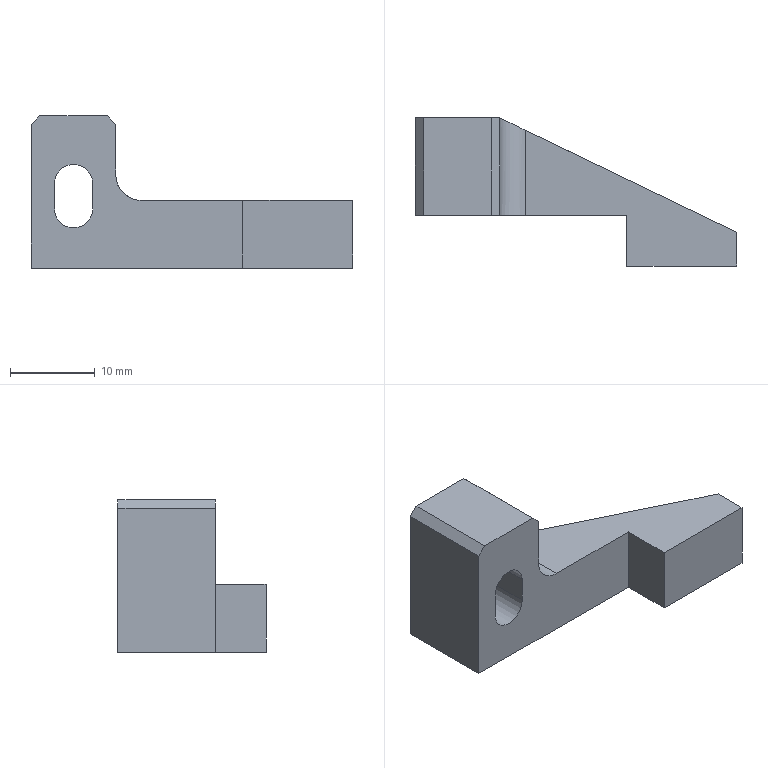Part | SolidWorks | features ICE 4, Chamfer 2, Extrusion 1, Fillet 1 | 1 solid | 25 faces | box 38 x 17.5 x 18 mm | volume 3099 mm3 | plane 19 | cylinder 6 | commonest cylinder face diameters 8 x3 4.5 x2 6 x1
STEP:
#1=CARTESIAN_POINT('',(5.,13.5,14.));
#2=VERTEX_POINT('',#1);
#3=CARTESIAN_POINT('',(9.,13.5,10.));
#4=VERTEX_POINT('',#3);
#5=CARTESIAN_POINT('',(5.,13.5,10.));
#6=DIRECTION('',(0.,1.,0.));
#7=DIRECTION('',(0.,0.,1.));
#8=AXIS2_PLACEMENT_3D('',#5,#6,#7);
#9=CIRCLE('',#8,4.);
#10=EDGE_CURVE('',#2,#4,#9,.T.);
#11=ORIENTED_EDGE('',*,*,#10,.F.);
#12=CARTESIAN_POINT('',(5.,17.5,14.));
#13=VERTEX_POINT('',#12);
#14=CARTESIAN_POINT('',(5.,13.5,14.));
#15=DIRECTION('',(0.,1.,0.));
#16=VECTOR('',#15,1000.);
#17=LINE('',#14,#16);
#18=EDGE_CURVE('',#2,#13,#17,.T.);
#19=ORIENTED_EDGE('',*,*,#18,.T.);
#20=CARTESIAN_POINT('',(9.,17.5,10.));
#21=VERTEX_POINT('',#20);
#22=CARTESIAN_POINT('',(5.,17.5,10.));
#23=DIRECTION('',(0.,1.,0.));
#24=DIRECTION('',(0.,0.,1.));
#25=AXIS2_PLACEMENT_3D('',#22,#23,#24);
#26=CIRCLE('',#25,4.);
#27=EDGE_CURVE('',#13,#21,#26,.T.);
#28=ORIENTED_EDGE('',*,*,#27,.T.);
#29=CARTESIAN_POINT('',(9.,13.5,10.));
#30=DIRECTION('',(0.,1.,0.));
#31=VECTOR('',#30,1000.);
#32=LINE('',#29,#31);
#33=EDGE_CURVE('',#4,#21,#32,.T.);
#34=ORIENTED_EDGE('',*,*,#33,.F.);
#35=EDGE_LOOP('',(#11,#19,#28,#34));
#36=FACE_OUTER_BOUND('',#35,.T.);
#37=CARTESIAN_POINT('',(5.,13.5,10.));
#38=DIRECTION('',(0.,1.,0.));
#39=DIRECTION('',(0.,0.,1.));
#40=AXIS2_PLACEMENT_3D('',#37,#38,#39);
#41=CYLINDRICAL_SURFACE('',#40,4.);
#42=ADVANCED_FACE('',(#36),#41,.F.);
#43=CARTESIAN_POINT('',(7.25,6.,10.));
#44=VERTEX_POINT('',#43);
#45=CARTESIAN_POINT('',(7.25,13.5,10.));
#46=VERTEX_POINT('',#45);
#47=CARTESIAN_POINT('',(7.25,-2.5,10.));
#48=DIRECTION('',(0.,1.,0.));
#49=VECTOR('',#48,1000.);
#50=LINE('',#47,#49);
#51=EDGE_CURVE('',#44,#46,#50,.T.);
#52=ORIENTED_EDGE('',*,*,#51,.F.);
#53=CARTESIAN_POINT('',(2.75,6.,10.));
#54=VERTEX_POINT('',#53);
#55=CARTESIAN_POINT('',(5.,6.,10.));
#56=DIRECTION('',(0.,-1.,0.));
#57=DIRECTION('',(0.,0.,1.));
#58=AXIS2_PLACEMENT_3D('',#55,#56,#57);
#59=CIRCLE('',#58,2.25);
#60=EDGE_CURVE('',#44,#54,#59,.T.);
#61=ORIENTED_EDGE('',*,*,#60,.T.);
#62=CARTESIAN_POINT('',(2.75,13.5,10.));
#63=VERTEX_POINT('',#62);
#64=CARTESIAN_POINT('',(2.75,-2.5,10.));
#65=DIRECTION('',(0.,1.,0.));
#66=VECTOR('',#65,1000.);
#67=LINE('',#64,#66);
#68=EDGE_CURVE('',#54,#63,#67,.T.);
#69=ORIENTED_EDGE('',*,*,#68,.T.);
#70=CARTESIAN_POINT('',(5.,13.5,10.));
#71=DIRECTION('',(0.,-1.,0.));
#72=DIRECTION('',(0.,0.,1.));
#73=AXIS2_PLACEMENT_3D('',#70,#71,#72);
#74=CIRCLE('',#73,2.25);
#75=EDGE_CURVE('',#46,#63,#74,.T.);
#76=ORIENTED_EDGE('',*,*,#75,.F.);
#77=EDGE_LOOP('',(#52,#61,#69,#76));
#78=FACE_OUTER_BOUND('',#77,.T.);
#79=CARTESIAN_POINT('',(5.,-2.5,10.));
#80=DIRECTION('',(0.,1.,0.));
#81=DIRECTION('',(-1.,0.,0.));
#82=AXIS2_PLACEMENT_3D('',#79,#80,#81);
#83=CYLINDRICAL_SURFACE('',#82,2.25);
#84=ADVANCED_FACE('',(#78),#83,.F.);
#85=ORIENTED_EDGE('',*,*,#68,.F.);
#86=CARTESIAN_POINT('',(2.75,6.,7.));
#87=VERTEX_POINT('',#86);
#88=CARTESIAN_POINT('',(2.75,6.,10.));
#89=DIRECTION('',(0.,0.,-1.));
#90=VECTOR('',#89,1000.);
#91=LINE('',#88,#90);
#92=EDGE_CURVE('',#54,#87,#91,.T.);
#93=ORIENTED_EDGE('',*,*,#92,.T.);
#94=CARTESIAN_POINT('',(2.75,13.5,7.));
#95=VERTEX_POINT('',#94);
#96=CARTESIAN_POINT('',(2.75,-2.5,7.));
#97=DIRECTION('',(0.,1.,0.));
#98=VECTOR('',#97,1000.);
#99=LINE('',#96,#98);
#100=EDGE_CURVE('',#87,#95,#99,.T.);
#101=ORIENTED_EDGE('',*,*,#100,.T.);
#102=CARTESIAN_POINT('',(2.75,13.5,10.));
#103=DIRECTION('',(0.,0.,-1.));
#104=VECTOR('',#103,1000.);
#105=LINE('',#102,#104);
#106=EDGE_CURVE('',#63,#95,#105,.T.);
#107=ORIENTED_EDGE('',*,*,#106,.F.);
#108=EDGE_LOOP('',(#85,#93,#101,#107));
#109=FACE_OUTER_BOUND('',#108,.T.);
#110=CARTESIAN_POINT('',(2.75,-2.5,10.));
#111=DIRECTION('',(-1.,0.,0.));
#112=DIRECTION('',(0.,-1.,0.));
#113=AXIS2_PLACEMENT_3D('',#110,#111,#112);
#114=PLANE('',#113);
#115=ADVANCED_FACE('',(#109),#114,.F.);
#116=ORIENTED_EDGE('',*,*,#100,.F.);
#117=CARTESIAN_POINT('',(7.25,6.,7.));
#118=VERTEX_POINT('',#117);
#119=CARTESIAN_POINT('',(5.,6.,7.));
#120=DIRECTION('',(0.,-1.,0.));
#121=DIRECTION('',(0.,0.,1.));
#122=AXIS2_PLACEMENT_3D('',#119,#120,#121);
#123=CIRCLE('',#122,2.25);
#124=EDGE_CURVE('',#87,#118,#123,.T.);
#125=ORIENTED_EDGE('',*,*,#124,.T.);
#126=CARTESIAN_POINT('',(7.25,13.5,7.));
#127=VERTEX_POINT('',#126);
#128=CARTESIAN_POINT('',(7.25,-2.5,7.));
#129=DIRECTION('',(0.,1.,0.));
#130=VECTOR('',#129,1000.);
#131=LINE('',#128,#130);
#132=EDGE_CURVE('',#118,#127,#131,.T.);
#133=ORIENTED_EDGE('',*,*,#132,.T.);
#134=CARTESIAN_POINT('',(5.,13.5,7.));
#135=DIRECTION('',(0.,-1.,0.));
#136=DIRECTION('',(0.,0.,1.));
#137=AXIS2_PLACEMENT_3D('',#134,#135,#136);
#138=CIRCLE('',#137,2.25);
#139=EDGE_CURVE('',#95,#127,#138,.T.);
#140=ORIENTED_EDGE('',*,*,#139,.F.);
#141=EDGE_LOOP('',(#116,#125,#133,#140));
#142=FACE_OUTER_BOUND('',#141,.T.);
#143=CARTESIAN_POINT('',(5.,-2.5,7.));
#144=DIRECTION('',(0.,1.,0.));
#145=DIRECTION('',(-1.,0.,0.));
#146=AXIS2_PLACEMENT_3D('',#143,#144,#145);
#147=CYLINDRICAL_SURFACE('',#146,2.25);
#148=ADVANCED_FACE('',(#142),#147,.F.);
#149=ORIENTED_EDGE('',*,*,#132,.F.);
#150=CARTESIAN_POINT('',(7.25,6.,10.));
#151=DIRECTION('',(0.,0.,1.));
#152=VECTOR('',#151,1000.);
#153=LINE('',#150,#152);
#154=EDGE_CURVE('',#118,#44,#153,.T.);
#155=ORIENTED_EDGE('',*,*,#154,.T.);
#156=ORIENTED_EDGE('',*,*,#51,.T.);
#157=CARTESIAN_POINT('',(7.25,13.5,10.));
#158=DIRECTION('',(0.,0.,1.));
#159=VECTOR('',#158,1000.);
#160=LINE('',#157,#159);
#161=EDGE_CURVE('',#127,#46,#160,.T.);
#162=ORIENTED_EDGE('',*,*,#161,.F.);
#163=EDGE_LOOP('',(#149,#155,#156,#162));
#164=FACE_OUTER_BOUND('',#163,.T.);
#165=CARTESIAN_POINT('',(7.25,-2.5,10.));
#166=DIRECTION('',(1.,0.,0.));
#167=DIRECTION('',(0.,1.,0.));
#168=AXIS2_PLACEMENT_3D('',#165,#166,#167);
#169=PLANE('',#168);
#170=ADVANCED_FACE('',(#164),#169,.F.);
#171=CARTESIAN_POINT('',(1.,17.5,7.));
#172=VERTEX_POINT('',#171);
#173=CARTESIAN_POINT('',(1.,17.5,10.));
#174=VERTEX_POINT('',#173);
#175=CARTESIAN_POINT('',(1.,17.5,7.));
#176=DIRECTION('',(0.,0.,1.));
#177=VECTOR('',#176,1000.);
#178=LINE('',#175,#177);
#179=EDGE_CURVE('',#172,#174,#178,.T.);
#180=ORIENTED_EDGE('',*,*,#179,.F.);
#181=CARTESIAN_POINT('',(9.,17.5,7.));
#182=VERTEX_POINT('',#181);
#183=CARTESIAN_POINT('',(5.,17.5,7.));
#184=DIRECTION('',(0.,1.,0.));
#185=DIRECTION('',(0.,0.,1.));
#186=AXIS2_PLACEMENT_3D('',#183,#184,#185);
#187=CIRCLE('',#186,4.);
#188=EDGE_CURVE('',#182,#172,#187,.T.);
#189=ORIENTED_EDGE('',*,*,#188,.F.);
#190=CARTESIAN_POINT('',(9.,17.5,7.));
#191=DIRECTION('',(0.,0.,-1.));
#192=VECTOR('',#191,1000.);
#193=LINE('',#190,#192);
#194=EDGE_CURVE('',#21,#182,#193,.T.);
#195=ORIENTED_EDGE('',*,*,#194,.F.);
#196=ORIENTED_EDGE('',*,*,#27,.F.);
#197=CARTESIAN_POINT('',(5.,17.5,10.));
#198=DIRECTION('',(0.,1.,0.));
#199=DIRECTION('',(0.,0.,1.));
#200=AXIS2_PLACEMENT_3D('',#197,#198,#199);
#201=CIRCLE('',#200,4.);
#202=EDGE_CURVE('',#174,#13,#201,.T.);
#203=ORIENTED_EDGE('',*,*,#202,.F.);
#204=EDGE_LOOP('',(#180,#189,#195,#196,#203));
#205=FACE_BOUND('',#204,.T.);
#206=CARTESIAN_POINT('',(9.,17.5,18.));
#207=VERTEX_POINT('',#206);
#208=CARTESIAN_POINT('',(1.,17.5,18.));
#209=VERTEX_POINT('',#208);
#210=CARTESIAN_POINT('',(10.,17.5,18.));
#211=DIRECTION('',(-1.,0.,0.));
#212=VECTOR('',#211,1000.);
#213=LINE('',#210,#212);
#214=EDGE_CURVE('',#207,#209,#213,.T.);
#215=ORIENTED_EDGE('',*,*,#214,.F.);
#216=CARTESIAN_POINT('',(10.,17.5,17.));
#217=VERTEX_POINT('',#216);
#218=CARTESIAN_POINT('',(9.,17.5,18.));
#219=DIRECTION('',(0.7071,0.,-0.7071));
#220=VECTOR('',#219,1000.);
#221=LINE('',#218,#220);
#222=EDGE_CURVE('',#207,#217,#221,.T.);
#223=ORIENTED_EDGE('',*,*,#222,.T.);
#224=CARTESIAN_POINT('',(10.,17.5,11.));
#225=VERTEX_POINT('',#224);
#226=CARTESIAN_POINT('',(10.,17.5,18.));
#227=DIRECTION('',(0.,0.,-1.));
#228=VECTOR('',#227,1000.);
#229=LINE('',#226,#228);
#230=EDGE_CURVE('',#217,#225,#229,.T.);
#231=ORIENTED_EDGE('',*,*,#230,.T.);
#232=CARTESIAN_POINT('',(10.,17.5,3.));
#233=VERTEX_POINT('',#232);
#234=CARTESIAN_POINT('',(10.,17.5,18.));
#235=DIRECTION('',(0.,0.,-1.));
#236=VECTOR('',#235,1000.);
#237=LINE('',#234,#236);
#238=EDGE_CURVE('',#225,#233,#237,.T.);
#239=ORIENTED_EDGE('',*,*,#238,.T.);
#240=CARTESIAN_POINT('',(3.092,17.5,0.));
#241=VERTEX_POINT('',#240);
#242=CARTESIAN_POINT('',(33.557,17.5,13.231));
#243=DIRECTION('',(-0.9172,0.,-0.3984));
#244=VECTOR('',#243,1000.);
#245=LINE('',#242,#244);
#246=EDGE_CURVE('',#233,#241,#245,.T.);
#247=ORIENTED_EDGE('',*,*,#246,.T.);
#248=CARTESIAN_POINT('',(0.,17.5,0.));
#249=VERTEX_POINT('',#248);
#250=CARTESIAN_POINT('',(10.,17.5,0.));
#251=DIRECTION('',(-1.,0.,0.));
#252=VECTOR('',#251,1000.);
#253=LINE('',#250,#252);
#254=EDGE_CURVE('',#241,#249,#253,.T.);
#255=ORIENTED_EDGE('',*,*,#254,.T.);
#256=CARTESIAN_POINT('',(0.,17.5,17.));
#257=VERTEX_POINT('',#256);
#258=CARTESIAN_POINT('',(0.,17.5,18.));
#259=DIRECTION('',(0.,0.,-1.));
#260=VECTOR('',#259,1000.);
#261=LINE('',#258,#260);
#262=EDGE_CURVE('',#257,#249,#261,.T.);
#263=ORIENTED_EDGE('',*,*,#262,.F.);
#264=CARTESIAN_POINT('',(1.,17.5,18.));
#265=DIRECTION('',(0.7071,0.,0.7071));
#266=VECTOR('',#265,1000.);
#267=LINE('',#264,#266);
#268=EDGE_CURVE('',#257,#209,#267,.T.);
#269=ORIENTED_EDGE('',*,*,#268,.T.);
#270=EDGE_LOOP('',(#215,#223,#231,#239,#247,#255,#263,#269));
#271=FACE_OUTER_BOUND('',#270,.T.);
#272=CARTESIAN_POINT('',(10.,17.5,18.));
#273=DIRECTION('',(0.,-1.,0.));
#274=DIRECTION('',(0.,0.,-1.));
#275=AXIS2_PLACEMENT_3D('',#272,#273,#274);
#276=PLANE('',#275);
#277=ADVANCED_FACE('',(#205,#271),#276,.F.);
#278=CARTESIAN_POINT('',(0.,6.,0.));
#279=VERTEX_POINT('',#278);
#280=CARTESIAN_POINT('',(0.,6.,17.));
#281=VERTEX_POINT('',#280);
#282=CARTESIAN_POINT('',(0.,6.,0.));
#283=DIRECTION('',(0.,0.,1.));
#284=VECTOR('',#283,1000.);
#285=LINE('',#282,#284);
#286=EDGE_CURVE('',#279,#281,#285,.T.);
#287=ORIENTED_EDGE('',*,*,#286,.T.);
#288=CARTESIAN_POINT('',(0.,17.5,17.));
#289=DIRECTION('',(0.,1.,0.));
#290=VECTOR('',#289,1000.);
#291=LINE('',#288,#290);
#292=EDGE_CURVE('',#281,#257,#291,.T.);
#293=ORIENTED_EDGE('',*,*,#292,.T.);
#294=ORIENTED_EDGE('',*,*,#262,.T.);
#295=CARTESIAN_POINT('',(0.,17.5,0.));
#296=DIRECTION('',(0.,-1.,0.));
#297=VECTOR('',#296,1000.);
#298=LINE('',#295,#297);
#299=EDGE_CURVE('',#249,#279,#298,.T.);
#300=ORIENTED_EDGE('',*,*,#299,.T.);
#301=EDGE_LOOP('',(#287,#293,#294,#300));
#302=FACE_OUTER_BOUND('',#301,.T.);
#303=CARTESIAN_POINT('',(0.,17.5,18.));
#304=DIRECTION('',(1.,0.,0.));
#305=DIRECTION('',(0.,1.,0.));
#306=AXIS2_PLACEMENT_3D('',#303,#304,#305);
#307=PLANE('',#306);
#308=ADVANCED_FACE('',(#302),#307,.F.);
#309=CARTESIAN_POINT('',(38.,0.,8.));
#310=VERTEX_POINT('',#309);
#311=CARTESIAN_POINT('',(38.,0.,0.));
#312=VERTEX_POINT('',#311);
#313=CARTESIAN_POINT('',(38.,0.,18.));
#314=DIRECTION('',(0.,0.,-1.));
#315=VECTOR('',#314,1000.);
#316=LINE('',#313,#315);
#317=EDGE_CURVE('',#310,#312,#316,.T.);
#318=ORIENTED_EDGE('',*,*,#317,.F.);
#319=CARTESIAN_POINT('',(25.,0.,8.));
#320=VERTEX_POINT('',#319);
#321=CARTESIAN_POINT('',(10.,0.,8.));
#322=DIRECTION('',(-1.,0.,0.));
#323=VECTOR('',#322,1000.);
#324=LINE('',#321,#323);
#325=EDGE_CURVE('',#310,#320,#324,.T.);
#326=ORIENTED_EDGE('',*,*,#325,.T.);
#327=CARTESIAN_POINT('',(25.,0.,0.));
#328=VERTEX_POINT('',#327);
#329=CARTESIAN_POINT('',(25.,0.,0.));
#330=DIRECTION('',(0.,0.,1.));
#331=VECTOR('',#330,1000.);
#332=LINE('',#329,#331);
#333=EDGE_CURVE('',#328,#320,#332,.T.);
#334=ORIENTED_EDGE('',*,*,#333,.F.);
#335=CARTESIAN_POINT('',(0.,0.,0.));
#336=DIRECTION('',(1.,0.,0.));
#337=VECTOR('',#336,1000.);
#338=LINE('',#335,#337);
#339=EDGE_CURVE('',#328,#312,#338,.T.);
#340=ORIENTED_EDGE('',*,*,#339,.T.);
#341=EDGE_LOOP('',(#318,#326,#334,#340));
#342=FACE_OUTER_BOUND('',#341,.T.);
#343=CARTESIAN_POINT('',(0.,0.,18.));
#344=DIRECTION('',(0.,1.,0.));
#345=DIRECTION('',(0.,0.,1.));
#346=AXIS2_PLACEMENT_3D('',#343,#344,#345);
#347=PLANE('',#346);
#348=ADVANCED_FACE('',(#342),#347,.F.);
#349=CARTESIAN_POINT('',(38.,4.,8.));
#350=VERTEX_POINT('',#349);
#351=CARTESIAN_POINT('',(38.,4.,3.));
#352=VERTEX_POINT('',#351);
#353=CARTESIAN_POINT('',(38.,4.,18.));
#354=DIRECTION('',(0.,0.,-1.));
#355=VECTOR('',#354,1000.);
#356=LINE('',#353,#355);
#357=EDGE_CURVE('',#350,#352,#356,.T.);
#358=ORIENTED_EDGE('',*,*,#357,.F.);
#359=CARTESIAN_POINT('',(38.,0.,8.));
#360=DIRECTION('',(0.,1.,0.));
#361=VECTOR('',#360,1000.);
#362=LINE('',#359,#361);
#363=EDGE_CURVE('',#310,#350,#362,.T.);
#364=ORIENTED_EDGE('',*,*,#363,.F.);
#365=ORIENTED_EDGE('',*,*,#317,.T.);
#366=CARTESIAN_POINT('',(38.,0.6695,0.));
#367=VERTEX_POINT('',#366);
#368=CARTESIAN_POINT('',(38.,0.,0.));
#369=DIRECTION('',(0.,1.,0.));
#370=VECTOR('',#369,1000.);
#371=LINE('',#368,#370);
#372=EDGE_CURVE('',#312,#367,#371,.T.);
#373=ORIENTED_EDGE('',*,*,#372,.T.);
#374=CARTESIAN_POINT('',(38.,4.,3.));
#375=DIRECTION('',(0.,0.743,0.6693));
#376=VECTOR('',#375,1000.);
#377=LINE('',#374,#376);
#378=EDGE_CURVE('',#367,#352,#377,.T.);
#379=ORIENTED_EDGE('',*,*,#378,.T.);
#380=EDGE_LOOP('',(#358,#364,#365,#373,#379));
#381=FACE_OUTER_BOUND('',#380,.T.);
#382=CARTESIAN_POINT('',(38.,0.,18.));
#383=DIRECTION('',(-1.,0.,0.));
#384=DIRECTION('',(0.,0.,1.));
#385=AXIS2_PLACEMENT_3D('',#382,#383,#384);
#386=PLANE('',#385);
#387=ADVANCED_FACE('',(#381),#386,.F.);
#388=ORIENTED_EDGE('',*,*,#238,.F.);
#389=CARTESIAN_POINT('',(13.,16.054,8.));
#390=VERTEX_POINT('',#389);
#391=CARTESIAN_POINT('',(10.,17.5,11.));
#392=CARTESIAN_POINT('',(10.,17.5,9.243));
#393=CARTESIAN_POINT('',(11.243,16.901,8.));
#394=CARTESIAN_POINT('',(13.,16.054,8.));
#395=(BOUNDED_CURVE()B_SPLINE_CURVE(3,(#391,#392,#393,#394),.UNSPECIFIED.,.F.,.F.)B_SPLINE_CURVE_WITH_KNOTS((4,4),(3.142,4.712),.UNSPECIFIED.)CURVE()GEOMETRIC_REPRESENTATION_ITEM()RATIONAL_B_SPLINE_CURVE((1.,0.8047,0.8047,1.))REPRESENTATION_ITEM(''));
#396=EDGE_CURVE('',#225,#390,#395,.T.);
#397=ORIENTED_EDGE('',*,*,#396,.T.);
#398=CARTESIAN_POINT('',(38.,4.,8.));
#399=DIRECTION('',(0.9008,-0.4343,0.));
#400=VECTOR('',#399,1000.);
#401=LINE('',#398,#400);
#402=EDGE_CURVE('',#390,#350,#401,.T.);
#403=ORIENTED_EDGE('',*,*,#402,.T.);
#404=ORIENTED_EDGE('',*,*,#357,.T.);
#405=CARTESIAN_POINT('',(38.,4.,3.));
#406=DIRECTION('',(-0.9008,0.4343,0.));
#407=VECTOR('',#406,1000.);
#408=LINE('',#405,#407);
#409=EDGE_CURVE('',#352,#233,#408,.T.);
#410=ORIENTED_EDGE('',*,*,#409,.T.);
#411=EDGE_LOOP('',(#388,#397,#403,#404,#410));
#412=FACE_OUTER_BOUND('',#411,.T.);
#413=CARTESIAN_POINT('',(38.,4.,18.));
#414=DIRECTION('',(-0.4343,-0.9008,0.));
#415=DIRECTION('',(0.9008,-0.4343,0.));
#416=AXIS2_PLACEMENT_3D('',#413,#414,#415);
#417=PLANE('',#416);
#418=ADVANCED_FACE('',(#412),#417,.F.);
#419=CARTESIAN_POINT('',(9.,6.,18.));
#420=VERTEX_POINT('',#419);
#421=CARTESIAN_POINT('',(1.,6.,18.));
#422=VERTEX_POINT('',#421);
#423=CARTESIAN_POINT('',(0.,6.,18.));
#424=DIRECTION('',(-1.,0.,0.));
#425=VECTOR('',#424,1000.);
#426=LINE('',#423,#425);
#427=EDGE_CURVE('',#420,#422,#426,.T.);
#428=ORIENTED_EDGE('',*,*,#427,.F.);
#429=CARTESIAN_POINT('',(9.,17.5,18.));
#430=DIRECTION('',(0.,1.,0.));
#431=VECTOR('',#430,1000.);
#432=LINE('',#429,#431);
#433=EDGE_CURVE('',#420,#207,#432,.T.);
#434=ORIENTED_EDGE('',*,*,#433,.T.);
#435=ORIENTED_EDGE('',*,*,#214,.T.);
#436=CARTESIAN_POINT('',(1.,6.,18.));
#437=DIRECTION('',(0.,-1.,0.));
#438=VECTOR('',#437,1000.);
#439=LINE('',#436,#438);
#440=EDGE_CURVE('',#209,#422,#439,.T.);
#441=ORIENTED_EDGE('',*,*,#440,.T.);
#442=EDGE_LOOP('',(#428,#434,#435,#441));
#443=FACE_OUTER_BOUND('',#442,.T.);
#444=CARTESIAN_POINT('',(0.,17.5,18.));
#445=DIRECTION('',(0.,0.,1.));
#446=DIRECTION('',(1.,0.,0.));
#447=AXIS2_PLACEMENT_3D('',#444,#445,#446);
#448=PLANE('',#447);
#449=ADVANCED_FACE('',(#443),#448,.T.);
#450=CARTESIAN_POINT('',(25.,6.,0.));
#451=VERTEX_POINT('',#450);
#452=CARTESIAN_POINT('',(25.,0.,0.));
#453=DIRECTION('',(0.,1.,0.));
#454=VECTOR('',#453,1000.);
#455=LINE('',#452,#454);
#456=EDGE_CURVE('',#328,#451,#455,.T.);
#457=ORIENTED_EDGE('',*,*,#456,.T.);
#458=CARTESIAN_POINT('',(0.,6.,0.));
#459=DIRECTION('',(-1.,0.,0.));
#460=VECTOR('',#459,1000.);
#461=LINE('',#458,#460);
#462=EDGE_CURVE('',#451,#279,#461,.T.);
#463=ORIENTED_EDGE('',*,*,#462,.T.);
#464=ORIENTED_EDGE('',*,*,#299,.F.);
#465=ORIENTED_EDGE('',*,*,#254,.F.);
#466=CARTESIAN_POINT('',(0.5833,18.71,0.));
#467=DIRECTION('',(0.9008,-0.4343,0.));
#468=VECTOR('',#467,1000.);
#469=LINE('',#466,#468);
#470=EDGE_CURVE('',#241,#367,#469,.T.);
#471=ORIENTED_EDGE('',*,*,#470,.T.);
#472=ORIENTED_EDGE('',*,*,#372,.F.);
#473=ORIENTED_EDGE('',*,*,#339,.F.);
#474=EDGE_LOOP('',(#457,#463,#464,#465,#471,#472,#473));
#475=FACE_OUTER_BOUND('',#474,.T.);
#476=CARTESIAN_POINT('',(0.,17.5,0.));
#477=DIRECTION('',(0.,0.,1.));
#478=DIRECTION('',(1.,0.,0.));
#479=AXIS2_PLACEMENT_3D('',#476,#477,#478);
#480=PLANE('',#479);
#481=ADVANCED_FACE('',(#475),#480,.F.);
#482=ORIENTED_EDGE('',*,*,#378,.F.);
#483=ORIENTED_EDGE('',*,*,#470,.F.);
#484=ORIENTED_EDGE('',*,*,#246,.F.);
#485=ORIENTED_EDGE('',*,*,#409,.F.);
#486=EDGE_LOOP('',(#482,#483,#484,#485));
#487=FACE_OUTER_BOUND('',#486,.T.);
#488=CARTESIAN_POINT('',(38.,4.,3.));
#489=DIRECTION('',(-0.3071,-0.6369,0.7071));
#490=DIRECTION('',(0.,-0.743,-0.6693));
#491=AXIS2_PLACEMENT_3D('',#488,#489,#490);
#492=PLANE('',#491);
#493=ADVANCED_FACE('',(#487),#492,.F.);
#494=CARTESIAN_POINT('',(9.,13.5,7.));
#495=VERTEX_POINT('',#494);
#496=CARTESIAN_POINT('',(1.,13.5,7.));
#497=VERTEX_POINT('',#496);
#498=CARTESIAN_POINT('',(5.,13.5,7.));
#499=DIRECTION('',(0.,1.,0.));
#500=DIRECTION('',(0.,0.,1.));
#501=AXIS2_PLACEMENT_3D('',#498,#499,#500);
#502=CIRCLE('',#501,4.);
#503=EDGE_CURVE('',#495,#497,#502,.T.);
#504=ORIENTED_EDGE('',*,*,#503,.T.);
#505=CARTESIAN_POINT('',(1.,13.5,10.));
#506=VERTEX_POINT('',#505);
#507=CARTESIAN_POINT('',(1.,13.5,7.));
#508=DIRECTION('',(0.,0.,1.));
#509=VECTOR('',#508,1000.);
#510=LINE('',#507,#509);
#511=EDGE_CURVE('',#497,#506,#510,.T.);
#512=ORIENTED_EDGE('',*,*,#511,.T.);
#513=CARTESIAN_POINT('',(5.,13.5,10.));
#514=DIRECTION('',(0.,1.,0.));
#515=DIRECTION('',(0.,0.,1.));
#516=AXIS2_PLACEMENT_3D('',#513,#514,#515);
#517=CIRCLE('',#516,4.);
#518=EDGE_CURVE('',#506,#2,#517,.T.);
#519=ORIENTED_EDGE('',*,*,#518,.T.);
#520=ORIENTED_EDGE('',*,*,#10,.T.);
#521=CARTESIAN_POINT('',(9.,13.5,7.));
#522=DIRECTION('',(0.,0.,-1.));
#523=VECTOR('',#522,1000.);
#524=LINE('',#521,#523);
#525=EDGE_CURVE('',#4,#495,#524,.T.);
#526=ORIENTED_EDGE('',*,*,#525,.T.);
#527=EDGE_LOOP('',(#504,#512,#519,#520,#526));
#528=FACE_OUTER_BOUND('',#527,.T.);
#529=ORIENTED_EDGE('',*,*,#75,.T.);
#530=ORIENTED_EDGE('',*,*,#106,.T.);
#531=ORIENTED_EDGE('',*,*,#139,.T.);
#532=ORIENTED_EDGE('',*,*,#161,.T.);
#533=EDGE_LOOP('',(#529,#530,#531,#532));
#534=FACE_BOUND('',#533,.T.);
#535=CARTESIAN_POINT('',(5.,13.5,7.));
#536=DIRECTION('',(0.,1.,0.));
#537=DIRECTION('',(0.,0.,1.));
#538=AXIS2_PLACEMENT_3D('',#535,#536,#537);
#539=PLANE('',#538);
#540=ADVANCED_FACE('',(#528,#534),#539,.T.);
#541=ORIENTED_EDGE('',*,*,#188,.T.);
#542=CARTESIAN_POINT('',(1.,13.5,7.));
#543=DIRECTION('',(0.,1.,0.));
#544=VECTOR('',#543,1000.);
#545=LINE('',#542,#544);
#546=EDGE_CURVE('',#497,#172,#545,.T.);
#547=ORIENTED_EDGE('',*,*,#546,.F.);
#548=ORIENTED_EDGE('',*,*,#503,.F.);
#549=CARTESIAN_POINT('',(9.,13.5,7.));
#550=DIRECTION('',(0.,1.,0.));
#551=VECTOR('',#550,1000.);
#552=LINE('',#549,#551);
#553=EDGE_CURVE('',#495,#182,#552,.T.);
#554=ORIENTED_EDGE('',*,*,#553,.T.);
#555=EDGE_LOOP('',(#541,#547,#548,#554));
#556=FACE_OUTER_BOUND('',#555,.T.);
#557=CARTESIAN_POINT('',(5.,13.5,7.));
#558=DIRECTION('',(0.,1.,0.));
#559=DIRECTION('',(0.,0.,1.));
#560=AXIS2_PLACEMENT_3D('',#557,#558,#559);
#561=CYLINDRICAL_SURFACE('',#560,4.);
#562=ADVANCED_FACE('',(#556),#561,.F.);
#563=ORIENTED_EDGE('',*,*,#194,.T.);
#564=ORIENTED_EDGE('',*,*,#553,.F.);
#565=ORIENTED_EDGE('',*,*,#525,.F.);
#566=ORIENTED_EDGE('',*,*,#33,.T.);
#567=EDGE_LOOP('',(#563,#564,#565,#566));
#568=FACE_OUTER_BOUND('',#567,.T.);
#569=CARTESIAN_POINT('',(9.,13.5,7.));
#570=DIRECTION('',(1.,0.,0.));
#571=DIRECTION('',(0.,0.,-1.));
#572=AXIS2_PLACEMENT_3D('',#569,#570,#571);
#573=PLANE('',#572);
#574=ADVANCED_FACE('',(#568),#573,.F.);
#575=ORIENTED_EDGE('',*,*,#18,.F.);
#576=ORIENTED_EDGE('',*,*,#518,.F.);
#577=CARTESIAN_POINT('',(1.,13.5,10.));
#578=DIRECTION('',(0.,1.,0.));
#579=VECTOR('',#578,1000.);
#580=LINE('',#577,#579);
#581=EDGE_CURVE('',#506,#174,#580,.T.);
#582=ORIENTED_EDGE('',*,*,#581,.T.);
#583=ORIENTED_EDGE('',*,*,#202,.T.);
#584=EDGE_LOOP('',(#575,#576,#582,#583));
#585=FACE_OUTER_BOUND('',#584,.T.);
#586=CARTESIAN_POINT('',(5.,13.5,10.));
#587=DIRECTION('',(0.,1.,0.));
#588=DIRECTION('',(0.,0.,1.));
#589=AXIS2_PLACEMENT_3D('',#586,#587,#588);
#590=CYLINDRICAL_SURFACE('',#589,4.);
#591=ADVANCED_FACE('',(#585),#590,.F.);
#592=ORIENTED_EDGE('',*,*,#179,.T.);
#593=ORIENTED_EDGE('',*,*,#581,.F.);
#594=ORIENTED_EDGE('',*,*,#511,.F.);
#595=ORIENTED_EDGE('',*,*,#546,.T.);
#596=EDGE_LOOP('',(#592,#593,#594,#595));
#597=FACE_OUTER_BOUND('',#596,.T.);
#598=CARTESIAN_POINT('',(1.,13.5,7.));
#599=DIRECTION('',(-1.,0.,0.));
#600=DIRECTION('',(0.,0.,1.));
#601=AXIS2_PLACEMENT_3D('',#598,#599,#600);
#602=PLANE('',#601);
#603=ADVANCED_FACE('',(#597),#602,.F.);
#604=CARTESIAN_POINT('',(10.,6.,11.));
#605=VERTEX_POINT('',#604);
#606=CARTESIAN_POINT('',(10.,6.,17.));
#607=VERTEX_POINT('',#606);
#608=CARTESIAN_POINT('',(10.,6.,0.));
#609=DIRECTION('',(0.,0.,1.));
#610=VECTOR('',#609,1000.);
#611=LINE('',#608,#610);
#612=EDGE_CURVE('',#605,#607,#611,.T.);
#613=ORIENTED_EDGE('',*,*,#612,.T.);
#614=CARTESIAN_POINT('',(9.,6.,18.));
#615=DIRECTION('',(-0.7071,0.,0.7071));
#616=VECTOR('',#615,1000.);
#617=LINE('',#614,#616);
#618=EDGE_CURVE('',#607,#420,#617,.T.);
#619=ORIENTED_EDGE('',*,*,#618,.T.);
#620=ORIENTED_EDGE('',*,*,#427,.T.);
#621=CARTESIAN_POINT('',(1.,6.,18.));
#622=DIRECTION('',(-0.7071,0.,-0.7071));
#623=VECTOR('',#622,1000.);
#624=LINE('',#621,#623);
#625=EDGE_CURVE('',#422,#281,#624,.T.);
#626=ORIENTED_EDGE('',*,*,#625,.T.);
#627=ORIENTED_EDGE('',*,*,#286,.F.);
#628=ORIENTED_EDGE('',*,*,#462,.F.);
#629=CARTESIAN_POINT('',(25.,6.,8.));
#630=VERTEX_POINT('',#629);
#631=CARTESIAN_POINT('',(25.,6.,0.));
#632=DIRECTION('',(0.,0.,1.));
#633=VECTOR('',#632,1000.);
#634=LINE('',#631,#633);
#635=EDGE_CURVE('',#451,#630,#634,.T.);
#636=ORIENTED_EDGE('',*,*,#635,.T.);
#637=CARTESIAN_POINT('',(13.,6.,8.));
#638=VERTEX_POINT('',#637);
#639=CARTESIAN_POINT('',(0.,6.,8.));
#640=DIRECTION('',(-1.,0.,0.));
#641=VECTOR('',#640,1000.);
#642=LINE('',#639,#641);
#643=EDGE_CURVE('',#630,#638,#642,.T.);
#644=ORIENTED_EDGE('',*,*,#643,.T.);
#645=CARTESIAN_POINT('',(13.,6.,11.));
#646=DIRECTION('',(0.,1.,0.));
#647=DIRECTION('',(0.,0.,1.));
#648=AXIS2_PLACEMENT_3D('',#645,#646,#647);
#649=CIRCLE('',#648,3.);
#650=EDGE_CURVE('',#638,#605,#649,.T.);
#651=ORIENTED_EDGE('',*,*,#650,.T.);
#652=EDGE_LOOP('',(#613,#619,#620,#626,#627,#628,#636,#644,#651));
#653=FACE_OUTER_BOUND('',#652,.T.);
#654=ORIENTED_EDGE('',*,*,#154,.F.);
#655=ORIENTED_EDGE('',*,*,#124,.F.);
#656=ORIENTED_EDGE('',*,*,#92,.F.);
#657=ORIENTED_EDGE('',*,*,#60,.F.);
#658=EDGE_LOOP('',(#654,#655,#656,#657));
#659=FACE_BOUND('',#658,.T.);
#660=CARTESIAN_POINT('',(0.,6.,0.));
#661=DIRECTION('',(0.,1.,0.));
#662=DIRECTION('',(0.,0.,1.));
#663=AXIS2_PLACEMENT_3D('',#660,#661,#662);
#664=PLANE('',#663);
#665=ADVANCED_FACE('',(#653,#659),#664,.F.);
#666=ORIENTED_EDGE('',*,*,#333,.T.);
#667=CARTESIAN_POINT('',(25.,0.,8.));
#668=DIRECTION('',(0.,1.,0.));
#669=VECTOR('',#668,1000.);
#670=LINE('',#667,#669);
#671=EDGE_CURVE('',#320,#630,#670,.T.);
#672=ORIENTED_EDGE('',*,*,#671,.T.);
#673=ORIENTED_EDGE('',*,*,#635,.F.);
#674=ORIENTED_EDGE('',*,*,#456,.F.);
#675=EDGE_LOOP('',(#666,#672,#673,#674));
#676=FACE_OUTER_BOUND('',#675,.T.);
#677=CARTESIAN_POINT('',(25.,0.,0.));
#678=DIRECTION('',(1.,0.,0.));
#679=DIRECTION('',(0.,0.,-1.));
#680=AXIS2_PLACEMENT_3D('',#677,#678,#679);
#681=PLANE('',#680);
#682=ADVANCED_FACE('',(#676),#681,.F.);
#683=ORIENTED_EDGE('',*,*,#230,.F.);
#684=CARTESIAN_POINT('',(10.,6.,17.));
#685=DIRECTION('',(0.,-1.,0.));
#686=VECTOR('',#685,1000.);
#687=LINE('',#684,#686);
#688=EDGE_CURVE('',#217,#607,#687,.T.);
#689=ORIENTED_EDGE('',*,*,#688,.T.);
#690=ORIENTED_EDGE('',*,*,#612,.F.);
#691=CARTESIAN_POINT('',(10.,17.5,11.));
#692=DIRECTION('',(0.,1.,0.));
#693=VECTOR('',#692,1000.);
#694=LINE('',#691,#693);
#695=EDGE_CURVE('',#605,#225,#694,.T.);
#696=ORIENTED_EDGE('',*,*,#695,.T.);
#697=EDGE_LOOP('',(#683,#689,#690,#696));
#698=FACE_OUTER_BOUND('',#697,.T.);
#699=CARTESIAN_POINT('',(10.,0.,18.));
#700=DIRECTION('',(-1.,0.,0.));
#701=DIRECTION('',(0.,0.,1.));
#702=AXIS2_PLACEMENT_3D('',#699,#700,#701);
#703=PLANE('',#702);
#704=ADVANCED_FACE('',(#698),#703,.F.);
#705=ORIENTED_EDGE('',*,*,#402,.F.);
#706=CARTESIAN_POINT('',(13.,6.,8.));
#707=DIRECTION('',(0.,-1.,0.));
#708=VECTOR('',#707,1000.);
#709=LINE('',#706,#708);
#710=EDGE_CURVE('',#390,#638,#709,.T.);
#711=ORIENTED_EDGE('',*,*,#710,.T.);
#712=ORIENTED_EDGE('',*,*,#643,.F.);
#713=ORIENTED_EDGE('',*,*,#671,.F.);
#714=ORIENTED_EDGE('',*,*,#325,.F.);
#715=ORIENTED_EDGE('',*,*,#363,.T.);
#716=EDGE_LOOP('',(#705,#711,#712,#713,#714,#715));
#717=FACE_OUTER_BOUND('',#716,.T.);
#718=CARTESIAN_POINT('',(10.,0.,8.));
#719=DIRECTION('',(0.,0.,-1.));
#720=DIRECTION('',(-1.,0.,0.));
#721=AXIS2_PLACEMENT_3D('',#718,#719,#720);
#722=PLANE('',#721);
#723=ADVANCED_FACE('',(#717),#722,.F.);
#724=ORIENTED_EDGE('',*,*,#650,.F.);
#725=ORIENTED_EDGE('',*,*,#710,.F.);
#726=ORIENTED_EDGE('',*,*,#396,.F.);
#727=ORIENTED_EDGE('',*,*,#695,.F.);
#728=EDGE_LOOP('',(#724,#725,#726,#727));
#729=FACE_OUTER_BOUND('',#728,.T.);
#730=CARTESIAN_POINT('',(13.,0.,11.));
#731=DIRECTION('',(0.,-1.,0.));
#732=DIRECTION('',(0.,0.,-1.));
#733=AXIS2_PLACEMENT_3D('',#730,#731,#732);
#734=CYLINDRICAL_SURFACE('',#733,3.);
#735=ADVANCED_FACE('',(#729),#734,.F.);
#736=ORIENTED_EDGE('',*,*,#618,.F.);
#737=ORIENTED_EDGE('',*,*,#688,.F.);
#738=ORIENTED_EDGE('',*,*,#222,.F.);
#739=ORIENTED_EDGE('',*,*,#433,.F.);
#740=EDGE_LOOP('',(#736,#737,#738,#739));
#741=FACE_OUTER_BOUND('',#740,.T.);
#742=CARTESIAN_POINT('',(9.,17.5,18.));
#743=DIRECTION('',(0.7071,0.,0.7071));
#744=DIRECTION('',(0.,-1.,0.));
#745=AXIS2_PLACEMENT_3D('',#742,#743,#744);
#746=PLANE('',#745);
#747=ADVANCED_FACE('',(#741),#746,.T.);
#748=ORIENTED_EDGE('',*,*,#268,.F.);
#749=ORIENTED_EDGE('',*,*,#292,.F.);
#750=ORIENTED_EDGE('',*,*,#625,.F.);
#751=ORIENTED_EDGE('',*,*,#440,.F.);
#752=EDGE_LOOP('',(#748,#749,#750,#751));
#753=FACE_OUTER_BOUND('',#752,.T.);
#754=CARTESIAN_POINT('',(1.,17.5,18.));
#755=DIRECTION('',(-0.7071,0.,0.7071));
#756=DIRECTION('',(0.,1.,0.));
#757=AXIS2_PLACEMENT_3D('',#754,#755,#756);
#758=PLANE('',#757);
#759=ADVANCED_FACE('',(#753),#758,.T.);
#760=CLOSED_SHELL('',(#42,#84,#115,#148,#170,#277,#308,#348,#387,#418,#449,#481,#493,#540,#562,#574,#591,#603,#665,#682,#704,#723,#735,#747,#759));
#761=MANIFOLD_SOLID_BREP('',#760);
#762=CARTESIAN_POINT('',(0.,0.,0.));
#763=DIRECTION('',(0.,0.,1.));
#764=DIRECTION('',(1.,0.,0.));
#765=AXIS2_PLACEMENT_3D('',#762,#763,#764);
#766=(LENGTH_UNIT()NAMED_UNIT(*)SI_UNIT(.MILLI.,.METRE.));
#767=UNCERTAINTY_MEASURE_WITH_UNIT(LENGTH_MEASURE(0.00001),#766,'','');
#768=(NAMED_UNIT(*)PLANE_ANGLE_UNIT()SI_UNIT($,.RADIAN.));
#769=(NAMED_UNIT(*)SI_UNIT($,.STERADIAN.)SOLID_ANGLE_UNIT());
#770=(GEOMETRIC_REPRESENTATION_CONTEXT(3)GLOBAL_UNCERTAINTY_ASSIGNED_CONTEXT((#767))GLOBAL_UNIT_ASSIGNED_CONTEXT((#766,#768,#769))REPRESENTATION_CONTEXT('',''));
#771=ADVANCED_BREP_SHAPE_REPRESENTATION('',(#761,#765),#770);